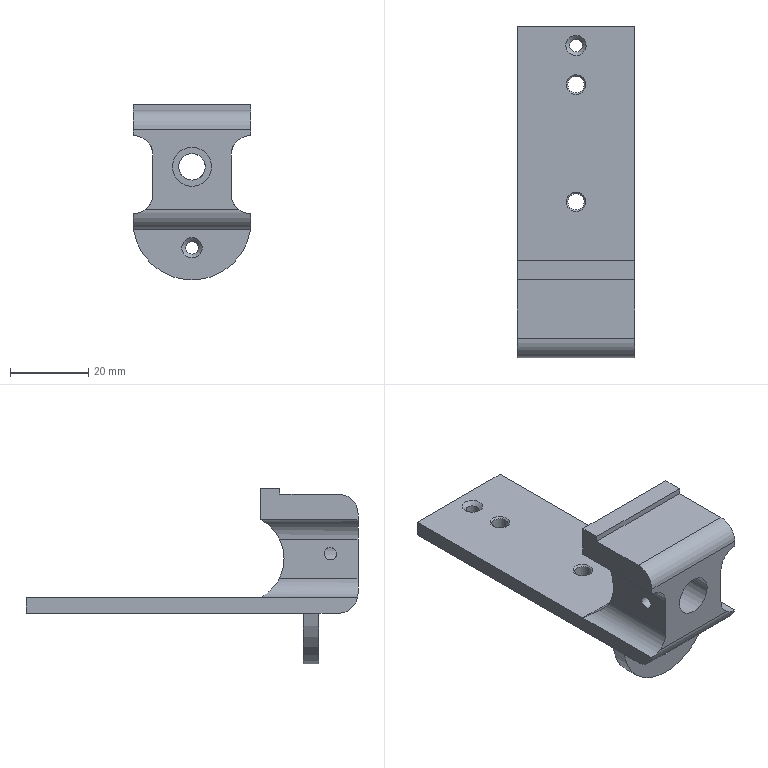Part | NX | features SKETCH 12, EXTRUDE 11, Linear Dimension 2, SIMPLE HOLE 2, SYMBOLIC_THREAD 2, BLEND 1, CHAMFER 1, DATUM_CSYS 1, HOLE PACKAGE 1 | 1 solid | 39 faces | box 30 x 85 x 45 mm | volume 23577 mm3 | plane 18 | cylinder 15 | cone 6 | commonest cylinder face diameters 10 x7 3.2 x3 4.2 x2 6.8 x1 22.545 x1 30.308 x1
STEP:
#1=CARTESIAN_POINT('',(-10.,20.1,-6.25));
#2=VERTEX_POINT('',#1);
#3=CARTESIAN_POINT('',(-10.,20.1,3.75));
#4=VERTEX_POINT('',#3);
#5=CARTESIAN_POINT('',(-10.,30.203,-1.25));
#6=DIRECTION('',(1.,0.,0.));
#7=DIRECTION('',(0.,0.,-1.));
#8=AXIS2_PLACEMENT_3D('',#5,#6,#7);
#9=CIRCLE('',#8,11.273);
#10=EDGE_CURVE('',#2,#4,#9,.F.);
#11=ORIENTED_EDGE('',*,*,#10,.F.);
#12=CARTESIAN_POINT('',(-10.,0.,-6.25));
#13=VERTEX_POINT('',#12);
#14=CARTESIAN_POINT('',(-10.,85.,-6.25));
#15=DIRECTION('',(0.,-1.,0.));
#16=VECTOR('',#15,1000.);
#17=LINE('',#14,#16);
#18=EDGE_CURVE('',#2,#13,#17,.T.);
#19=ORIENTED_EDGE('',*,*,#18,.T.);
#20=CARTESIAN_POINT('',(-10.,0.,3.75));
#21=VERTEX_POINT('',#20);
#22=CARTESIAN_POINT('',(-10.,0.,-6.25));
#23=DIRECTION('',(0.,0.,1.));
#24=VECTOR('',#23,1000.);
#25=LINE('',#22,#24);
#26=EDGE_CURVE('',#13,#21,#25,.T.);
#27=ORIENTED_EDGE('',*,*,#26,.T.);
#28=CARTESIAN_POINT('',(-10.,85.,3.75));
#29=DIRECTION('',(0.,-1.,0.));
#30=VECTOR('',#29,1000.);
#31=LINE('',#28,#30);
#32=EDGE_CURVE('',#4,#21,#31,.T.);
#33=ORIENTED_EDGE('',*,*,#32,.F.);
#34=EDGE_LOOP('',(#11,#19,#27,#33));
#35=FACE_BOUND('',#34,.T.);
#36=CARTESIAN_POINT('',(-10.,5.47,0.));
#37=VERTEX_POINT('',#36);
#38=CARTESIAN_POINT('',(-10.,7.07,0.));
#39=DIRECTION('',(-1.,0.,0.));
#40=DIRECTION('',(0.,-1.,0.));
#41=AXIS2_PLACEMENT_3D('',#38,#39,#40);
#42=CIRCLE('',#41,1.6);
#43=EDGE_CURVE('',#37,#37,#42,.T.);
#44=ORIENTED_EDGE('',*,*,#43,.F.);
#45=EDGE_LOOP('',(#44));
#46=FACE_BOUND('',#45,.T.);
#47=CARTESIAN_POINT('',(-10.,85.,-6.25));
#48=DIRECTION('',(1.,0.,0.));
#49=DIRECTION('',(0.,0.,-1.));
#50=AXIS2_PLACEMENT_3D('',#47,#48,#49);
#51=PLANE('',#50);
#52=ADVANCED_FACE('',(#35,#46),#51,.F.);
#53=CARTESIAN_POINT('',(5.,0.,0.75));
#54=VERTEX_POINT('',#53);
#55=CARTESIAN_POINT('',(0.,0.,0.75));
#56=DIRECTION('',(0.,-1.,0.));
#57=DIRECTION('',(1.,0.,0.));
#58=AXIS2_PLACEMENT_3D('',#55,#56,#57);
#59=CIRCLE('',#58,5.);
#60=EDGE_CURVE('',#54,#54,#59,.T.);
#61=ORIENTED_EDGE('',*,*,#60,.T.);
#62=EDGE_LOOP('',(#61));
#63=FACE_BOUND('',#62,.T.);
#64=CARTESIAN_POINT('',(5.,10.,0.75));
#65=VERTEX_POINT('',#64);
#66=CARTESIAN_POINT('',(0.,10.,0.75));
#67=DIRECTION('',(0.,-1.,0.));
#68=DIRECTION('',(1.,0.,0.));
#69=AXIS2_PLACEMENT_3D('',#66,#67,#68);
#70=CIRCLE('',#69,5.);
#71=EDGE_CURVE('',#65,#65,#70,.T.);
#72=ORIENTED_EDGE('',*,*,#71,.F.);
#73=EDGE_LOOP('',(#72));
#74=FACE_BOUND('',#73,.T.);
#75=CARTESIAN_POINT('',(-4.413,7.07,-1.6));
#76=VERTEX_POINT('',#75);
#77=CARTESIAN_POINT('',(-4.618,8.317,-1.249));
#78=CARTESIAN_POINT('',(-4.311,7.07,-1.776));
#79=CARTESIAN_POINT('',(-4.618,5.821,-1.248));
#80=CARTESIAN_POINT('',(-5.002,5.3,-0.04411));
#81=CARTESIAN_POINT('',(-5.007,5.799,1.248));
#82=CARTESIAN_POINT('',(-4.887,7.069,1.776));
#83=CARTESIAN_POINT('',(-5.007,8.34,1.248));
#84=CARTESIAN_POINT('',(-5.002,8.84,-0.04285));
#85=CARTESIAN_POINT('',(-4.618,8.317,-1.249));
#86=CARTESIAN_POINT('',(-4.311,7.07,-1.776));
#87=CARTESIAN_POINT('',(-4.618,5.821,-1.248));
#88=B_SPLINE_CURVE_WITH_KNOTS('',3,(#77,#78,#79,#80,#81,#82,#83,#84,#85,#86,#87),.UNSPECIFIED.,.T.,.F.,(1,1,1,1,1,1,1,1,1,1,1,1,1,1,1),(-0.003801,-0.002534,-0.001267,0.,0.001267,0.002534,0.003801,0.005068,0.006335,0.007602,0.008869,0.01014,0.0114,0.01267,0.01394),.UNSPECIFIED.);
#89=EDGE_CURVE('',#76,#76,#88,.T.);
#90=ORIENTED_EDGE('',*,*,#89,.T.);
#91=EDGE_LOOP('',(#90));
#92=FACE_BOUND('',#91,.T.);
#93=CARTESIAN_POINT('',(0.,10.,0.75));
#94=DIRECTION('',(0.,-1.,0.));
#95=DIRECTION('',(0.,0.,-1.));
#96=AXIS2_PLACEMENT_3D('',#93,#94,#95);
#97=CYLINDRICAL_SURFACE('',#96,5.);
#98=ADVANCED_FACE('',(#63,#74,#92),#97,.F.);
#99=CARTESIAN_POINT('',(15.,25.,8.75));
#100=VERTEX_POINT('',#99);
#101=CARTESIAN_POINT('',(15.,25.,16.75));
#102=VERTEX_POINT('',#101);
#103=CARTESIAN_POINT('',(15.,25.,-11.25));
#104=DIRECTION('',(0.,0.,1.));
#105=VECTOR('',#104,1000.);
#106=LINE('',#103,#105);
#107=EDGE_CURVE('',#100,#102,#106,.T.);
#108=ORIENTED_EDGE('',*,*,#107,.F.);
#109=CARTESIAN_POINT('',(-15.,25.,8.75));
#110=VERTEX_POINT('',#109);
#111=CARTESIAN_POINT('',(-18.,25.,8.75));
#112=DIRECTION('',(1.,0.,0.));
#113=VECTOR('',#112,1000.);
#114=LINE('',#111,#113);
#115=EDGE_CURVE('',#110,#100,#114,.T.);
#116=ORIENTED_EDGE('',*,*,#115,.F.);
#117=CARTESIAN_POINT('',(-15.,25.,16.75));
#118=VERTEX_POINT('',#117);
#119=CARTESIAN_POINT('',(-15.,25.,16.75));
#120=DIRECTION('',(0.,0.,-1.));
#121=VECTOR('',#120,1000.);
#122=LINE('',#119,#121);
#123=EDGE_CURVE('',#118,#110,#122,.T.);
#124=ORIENTED_EDGE('',*,*,#123,.F.);
#125=CARTESIAN_POINT('',(15.,25.,16.75));
#126=DIRECTION('',(-1.,0.,0.));
#127=VECTOR('',#126,1000.);
#128=LINE('',#125,#127);
#129=EDGE_CURVE('',#102,#118,#128,.T.);
#130=ORIENTED_EDGE('',*,*,#129,.F.);
#131=EDGE_LOOP('',(#108,#116,#124,#130));
#132=FACE_BOUND('',#131,.T.);
#133=CARTESIAN_POINT('',(-18.,25.,-11.25));
#134=DIRECTION('',(0.,1.,0.));
#135=DIRECTION('',(0.,0.,1.));
#136=AXIS2_PLACEMENT_3D('',#133,#134,#135);
#137=PLANE('',#136);
#138=ADVANCED_FACE('',(#132),#137,.T.);
#139=CARTESIAN_POINT('',(10.,20.1,3.75));
#140=VERTEX_POINT('',#139);
#141=CARTESIAN_POINT('',(10.,0.,3.75));
#142=VERTEX_POINT('',#141);
#143=CARTESIAN_POINT('',(10.,85.,3.75));
#144=DIRECTION('',(0.,-1.,0.));
#145=VECTOR('',#144,1000.);
#146=LINE('',#143,#145);
#147=EDGE_CURVE('',#140,#142,#146,.T.);
#148=ORIENTED_EDGE('',*,*,#147,.F.);
#149=CARTESIAN_POINT('',(10.,20.1,3.75));
#150=CARTESIAN_POINT('',(10.,20.45,4.457));
#151=CARTESIAN_POINT('',(10.293,21.285,5.764));
#152=CARTESIAN_POINT('',(11.33,22.76,7.294));
#153=CARTESIAN_POINT('',(12.777,24.25,8.368));
#154=CARTESIAN_POINT('',(14.204,25.,8.75));
#155=CARTESIAN_POINT('',(15.,25.,8.75));
#156=B_SPLINE_CURVE_WITH_KNOTS('',3,(#149,#150,#151,#152,#153,#154,#155),.UNSPECIFIED.,.F.,.F.,(4,1,1,1,4),(0.,0.002329,0.004658,0.006987,0.009316),.UNSPECIFIED.);
#157=EDGE_CURVE('',#140,#100,#156,.T.);
#158=ORIENTED_EDGE('',*,*,#157,.T.);
#159=CARTESIAN_POINT('',(15.,0.,8.75));
#160=VERTEX_POINT('',#159);
#161=CARTESIAN_POINT('',(15.,85.,8.75));
#162=DIRECTION('',(0.,-1.,0.));
#163=VECTOR('',#162,1000.);
#164=LINE('',#161,#163);
#165=EDGE_CURVE('',#100,#160,#164,.T.);
#166=ORIENTED_EDGE('',*,*,#165,.T.);
#167=CARTESIAN_POINT('',(15.,0.,3.75));
#168=DIRECTION('',(0.,1.,0.));
#169=DIRECTION('',(1.,0.,0.));
#170=AXIS2_PLACEMENT_3D('',#167,#168,#169);
#171=CIRCLE('',#170,5.);
#172=EDGE_CURVE('',#142,#160,#171,.T.);
#173=ORIENTED_EDGE('',*,*,#172,.F.);
#174=EDGE_LOOP('',(#148,#158,#166,#173));
#175=FACE_BOUND('',#174,.T.);
#176=CARTESIAN_POINT('',(15.,85.,3.75));
#177=DIRECTION('',(0.,-1.,0.));
#178=DIRECTION('',(0.,0.,-1.));
#179=AXIS2_PLACEMENT_3D('',#176,#177,#178);
#180=CYLINDRICAL_SURFACE('',#179,5.);
#181=ADVANCED_FACE('',(#175),#180,.F.);
#182=CARTESIAN_POINT('',(15.,25.,-11.25));
#183=VERTEX_POINT('',#182);
#184=CARTESIAN_POINT('',(15.,0.101,-11.25));
#185=VERTEX_POINT('',#184);
#186=CARTESIAN_POINT('',(15.,85.,-11.25));
#187=DIRECTION('',(0.,-1.,0.));
#188=VECTOR('',#187,1000.);
#189=LINE('',#186,#188);
#190=EDGE_CURVE('',#183,#185,#189,.T.);
#191=ORIENTED_EDGE('',*,*,#190,.F.);
#192=CARTESIAN_POINT('',(10.,20.1,-6.25));
#193=VERTEX_POINT('',#192);
#194=CARTESIAN_POINT('',(15.,25.,-11.25));
#195=CARTESIAN_POINT('',(14.207,25.,-11.25));
#196=CARTESIAN_POINT('',(12.784,24.255,-10.871));
#197=CARTESIAN_POINT('',(11.33,22.76,-9.795));
#198=CARTESIAN_POINT('',(10.293,21.284,-8.264));
#199=CARTESIAN_POINT('',(10.,20.449,-6.955));
#200=CARTESIAN_POINT('',(10.,20.1,-6.25));
#201=B_SPLINE_CURVE_WITH_KNOTS('',3,(#194,#195,#196,#197,#198,#199,#200),.UNSPECIFIED.,.F.,.F.,(4,1,1,1,4),(0.,0.002339,0.004679,0.007018,0.009357),.UNSPECIFIED.);
#202=EDGE_CURVE('',#183,#193,#201,.T.);
#203=ORIENTED_EDGE('',*,*,#202,.T.);
#204=CARTESIAN_POINT('',(10.,0.,-6.25));
#205=VERTEX_POINT('',#204);
#206=CARTESIAN_POINT('',(10.,85.,-6.25));
#207=DIRECTION('',(0.,-1.,0.));
#208=VECTOR('',#207,1000.);
#209=LINE('',#206,#208);
#210=EDGE_CURVE('',#193,#205,#209,.T.);
#211=ORIENTED_EDGE('',*,*,#210,.T.);
#212=CARTESIAN_POINT('',(12.,0.,-10.25));
#213=VERTEX_POINT('',#212);
#214=CARTESIAN_POINT('',(15.,0.,-6.25));
#215=DIRECTION('',(0.,1.,0.));
#216=DIRECTION('',(1.,0.,0.));
#217=AXIS2_PLACEMENT_3D('',#214,#215,#216);
#218=CIRCLE('',#217,5.);
#219=EDGE_CURVE('',#213,#205,#218,.T.);
#220=ORIENTED_EDGE('',*,*,#219,.F.);
#221=CARTESIAN_POINT('',(12.,0.,-10.25));
#222=CARTESIAN_POINT('',(12.867,0.,-10.9));
#223=CARTESIAN_POINT('',(13.917,0.101,-11.25));
#224=CARTESIAN_POINT('',(15.,0.101,-11.25));
#225=B_SPLINE_CURVE_WITH_KNOTS('',3,(#221,#222,#223,#224),.UNSPECIFIED.,.F.,.F.,(4,4),(0.,0.003202),.UNSPECIFIED.);
#226=EDGE_CURVE('',#213,#185,#225,.T.);
#227=ORIENTED_EDGE('',*,*,#226,.T.);
#228=EDGE_LOOP('',(#191,#203,#211,#220,#227));
#229=FACE_BOUND('',#228,.T.);
#230=CARTESIAN_POINT('',(15.,85.,-6.25));
#231=DIRECTION('',(0.,-1.,0.));
#232=DIRECTION('',(0.,0.,-1.));
#233=AXIS2_PLACEMENT_3D('',#230,#231,#232);
#234=CYLINDRICAL_SURFACE('',#233,5.);
#235=ADVANCED_FACE('',(#229),#234,.F.);
#236=ORIENTED_EDGE('',*,*,#210,.F.);
#237=CARTESIAN_POINT('',(10.,30.203,-1.25));
#238=DIRECTION('',(1.,0.,0.));
#239=DIRECTION('',(0.,0.,-1.));
#240=AXIS2_PLACEMENT_3D('',#237,#238,#239);
#241=CIRCLE('',#240,11.273);
#242=EDGE_CURVE('',#193,#140,#241,.F.);
#243=ORIENTED_EDGE('',*,*,#242,.T.);
#244=ORIENTED_EDGE('',*,*,#147,.T.);
#245=CARTESIAN_POINT('',(10.,0.,-6.25));
#246=DIRECTION('',(0.,0.,1.));
#247=VECTOR('',#246,1000.);
#248=LINE('',#245,#247);
#249=EDGE_CURVE('',#205,#142,#248,.T.);
#250=ORIENTED_EDGE('',*,*,#249,.F.);
#251=EDGE_LOOP('',(#236,#243,#244,#250));
#252=FACE_BOUND('',#251,.T.);
#253=CARTESIAN_POINT('',(10.,85.,-6.25));
#254=DIRECTION('',(1.,0.,0.));
#255=DIRECTION('',(0.,0.,-1.));
#256=AXIS2_PLACEMENT_3D('',#253,#254,#255);
#257=PLANE('',#256);
#258=ADVANCED_FACE('',(#252),#257,.T.);
#259=CARTESIAN_POINT('',(-15.,25.,-11.25));
#260=VERTEX_POINT('',#259);
#261=CARTESIAN_POINT('',(-15.,25.,-11.25));
#262=CARTESIAN_POINT('',(-14.207,25.,-11.25));
#263=CARTESIAN_POINT('',(-12.784,24.255,-10.871));
#264=CARTESIAN_POINT('',(-11.33,22.76,-9.795));
#265=CARTESIAN_POINT('',(-10.293,21.284,-8.264));
#266=CARTESIAN_POINT('',(-10.,20.449,-6.955));
#267=CARTESIAN_POINT('',(-10.,20.1,-6.25));
#268=B_SPLINE_CURVE_WITH_KNOTS('',3,(#261,#262,#263,#264,#265,#266,#267),.UNSPECIFIED.,.F.,.F.,(4,1,1,1,4),(0.,0.002339,0.004679,0.007018,0.009357),.UNSPECIFIED.);
#269=EDGE_CURVE('',#260,#2,#268,.T.);
#270=ORIENTED_EDGE('',*,*,#269,.F.);
#271=CARTESIAN_POINT('',(-15.,0.101,-11.25));
#272=VERTEX_POINT('',#271);
#273=CARTESIAN_POINT('',(-15.,85.,-11.25));
#274=DIRECTION('',(0.,-1.,0.));
#275=VECTOR('',#274,1000.);
#276=LINE('',#273,#275);
#277=EDGE_CURVE('',#260,#272,#276,.T.);
#278=ORIENTED_EDGE('',*,*,#277,.T.);
#279=CARTESIAN_POINT('',(-12.,0.,-10.25));
#280=VERTEX_POINT('',#279);
#281=CARTESIAN_POINT('',(-15.,0.101,-11.25));
#282=CARTESIAN_POINT('',(-13.917,0.101,-11.25));
#283=CARTESIAN_POINT('',(-12.866,0.,-10.9));
#284=CARTESIAN_POINT('',(-12.,0.,-10.25));
#285=B_SPLINE_CURVE_WITH_KNOTS('',3,(#281,#282,#283,#284),.UNSPECIFIED.,.F.,.F.,(4,4),(0.,0.003201),.UNSPECIFIED.);
#286=EDGE_CURVE('',#272,#280,#285,.T.);
#287=ORIENTED_EDGE('',*,*,#286,.T.);
#288=CARTESIAN_POINT('',(-15.,0.,-6.25));
#289=DIRECTION('',(0.,-1.,0.));
#290=DIRECTION('',(1.,0.,0.));
#291=AXIS2_PLACEMENT_3D('',#288,#289,#290);
#292=CIRCLE('',#291,5.);
#293=EDGE_CURVE('',#280,#13,#292,.T.);
#294=ORIENTED_EDGE('',*,*,#293,.T.);
#295=ORIENTED_EDGE('',*,*,#18,.F.);
#296=EDGE_LOOP('',(#270,#278,#287,#294,#295));
#297=FACE_BOUND('',#296,.T.);
#298=CARTESIAN_POINT('',(-15.,85.,-6.25));
#299=DIRECTION('',(0.,-1.,0.));
#300=DIRECTION('',(0.,0.,-1.));
#301=AXIS2_PLACEMENT_3D('',#298,#299,#300);
#302=CYLINDRICAL_SURFACE('',#301,5.);
#303=ADVANCED_FACE('',(#297),#302,.F.);
#304=CARTESIAN_POINT('',(-10.,20.1,3.75));
#305=CARTESIAN_POINT('',(-10.,20.45,4.457));
#306=CARTESIAN_POINT('',(-10.293,21.285,5.764));
#307=CARTESIAN_POINT('',(-11.33,22.76,7.294));
#308=CARTESIAN_POINT('',(-12.777,24.25,8.368));
#309=CARTESIAN_POINT('',(-14.204,25.,8.75));
#310=CARTESIAN_POINT('',(-15.,25.,8.75));
#311=B_SPLINE_CURVE_WITH_KNOTS('',3,(#304,#305,#306,#307,#308,#309,#310),.UNSPECIFIED.,.F.,.F.,(4,1,1,1,4),(0.,0.002329,0.004658,0.006987,0.009316),.UNSPECIFIED.);
#312=EDGE_CURVE('',#4,#110,#311,.T.);
#313=ORIENTED_EDGE('',*,*,#312,.F.);
#314=ORIENTED_EDGE('',*,*,#32,.T.);
#315=CARTESIAN_POINT('',(-15.,0.,8.75));
#316=VERTEX_POINT('',#315);
#317=CARTESIAN_POINT('',(-15.,0.,3.75));
#318=DIRECTION('',(0.,-1.,0.));
#319=DIRECTION('',(1.,0.,0.));
#320=AXIS2_PLACEMENT_3D('',#317,#318,#319);
#321=CIRCLE('',#320,5.);
#322=EDGE_CURVE('',#21,#316,#321,.T.);
#323=ORIENTED_EDGE('',*,*,#322,.T.);
#324=CARTESIAN_POINT('',(-15.,85.,8.75));
#325=DIRECTION('',(0.,-1.,0.));
#326=VECTOR('',#325,1000.);
#327=LINE('',#324,#326);
#328=EDGE_CURVE('',#110,#316,#327,.T.);
#329=ORIENTED_EDGE('',*,*,#328,.F.);
#330=EDGE_LOOP('',(#313,#314,#323,#329));
#331=FACE_BOUND('',#330,.T.);
#332=CARTESIAN_POINT('',(-15.,85.,3.75));
#333=DIRECTION('',(0.,-1.,0.));
#334=DIRECTION('',(0.,0.,-1.));
#335=AXIS2_PLACEMENT_3D('',#332,#333,#334);
#336=CYLINDRICAL_SURFACE('',#335,5.);
#337=ADVANCED_FACE('',(#331),#336,.F.);
#338=CARTESIAN_POINT('',(3.4,10.,0.75));
#339=VERTEX_POINT('',#338);
#340=CARTESIAN_POINT('',(0.,10.,0.75));
#341=DIRECTION('',(0.,-1.,0.));
#342=DIRECTION('',(1.,0.,0.));
#343=AXIS2_PLACEMENT_3D('',#340,#341,#342);
#344=CIRCLE('',#343,3.4);
#345=EDGE_CURVE('',#339,#339,#344,.T.);
#346=ORIENTED_EDGE('',*,*,#345,.T.);
#347=EDGE_LOOP('',(#346));
#348=FACE_BOUND('',#347,.T.);
#349=CARTESIAN_POINT('',(0.,19.018,-2.65));
#350=VERTEX_POINT('',#349);
#351=CARTESIAN_POINT('',(-2.712,18.885,-1.892));
#352=CARTESIAN_POINT('',(0.001244,19.084,-3.028));
#353=CARTESIAN_POINT('',(2.707,18.886,-1.894));
#354=CARTESIAN_POINT('',(3.759,18.994,0.8455));
#355=CARTESIAN_POINT('',(2.652,19.864,3.401));
#356=CARTESIAN_POINT('',(0.008689,20.53,4.524));
#357=CARTESIAN_POINT('',(-2.652,19.865,3.404));
#358=CARTESIAN_POINT('',(-3.758,18.996,0.8528));
#359=CARTESIAN_POINT('',(-2.712,18.885,-1.892));
#360=CARTESIAN_POINT('',(0.001244,19.084,-3.028));
#361=CARTESIAN_POINT('',(2.707,18.886,-1.894));
#362=B_SPLINE_CURVE_WITH_KNOTS('',3,(#351,#352,#353,#354,#355,#356,#357,#358,#359,#360,#361),.UNSPECIFIED.,.T.,.F.,(1,1,1,1,1,1,1,1,1,1,1,1,1,1,1),(-0.00809,-0.005393,-0.002697,0.,0.002697,0.005393,0.00809,0.01079,0.01348,0.01618,0.01888,0.02157,0.02427,0.02697,0.02966),.UNSPECIFIED.);
#363=EDGE_CURVE('',#350,#350,#362,.T.);
#364=ORIENTED_EDGE('',*,*,#363,.F.);
#365=EDGE_LOOP('',(#364));
#366=FACE_BOUND('',#365,.T.);
#367=CARTESIAN_POINT('',(0.,92.5,0.75));
#368=DIRECTION('',(0.,-1.,0.));
#369=DIRECTION('',(0.,0.,-1.));
#370=AXIS2_PLACEMENT_3D('',#367,#368,#369);
#371=CYLINDRICAL_SURFACE('',#370,3.4);
#372=ADVANCED_FACE('',(#348,#366),#371,.F.);
#373=CARTESIAN_POINT('',(15.,14.,-15.25));
#374=VERTEX_POINT('',#373);
#375=CARTESIAN_POINT('',(15.,10.,-15.25));
#376=VERTEX_POINT('',#375);
#377=CARTESIAN_POINT('',(15.,85.,-15.25));
#378=DIRECTION('',(0.,-1.,0.));
#379=VECTOR('',#378,1000.);
#380=LINE('',#377,#379);
#381=EDGE_CURVE('',#374,#376,#380,.T.);
#382=ORIENTED_EDGE('',*,*,#381,.T.);
#383=CARTESIAN_POINT('',(-15.,10.,-15.25));
#384=VERTEX_POINT('',#383);
#385=CARTESIAN_POINT('',(0.,10.,-13.096));
#386=DIRECTION('',(0.,-1.,0.));
#387=DIRECTION('',(0.,0.,-1.));
#388=AXIS2_PLACEMENT_3D('',#385,#386,#387);
#389=CIRCLE('',#388,15.154);
#390=EDGE_CURVE('',#376,#384,#389,.F.);
#391=ORIENTED_EDGE('',*,*,#390,.T.);
#392=CARTESIAN_POINT('',(-15.,14.,-15.25));
#393=VERTEX_POINT('',#392);
#394=CARTESIAN_POINT('',(-15.,85.,-15.25));
#395=DIRECTION('',(0.,-1.,0.));
#396=VECTOR('',#395,1000.);
#397=LINE('',#394,#396);
#398=EDGE_CURVE('',#393,#384,#397,.T.);
#399=ORIENTED_EDGE('',*,*,#398,.F.);
#400=CARTESIAN_POINT('',(0.,14.,-13.096));
#401=DIRECTION('',(0.,1.,0.));
#402=DIRECTION('',(0.,0.,1.));
#403=AXIS2_PLACEMENT_3D('',#400,#401,#402);
#404=CIRCLE('',#403,15.154);
#405=EDGE_CURVE('',#393,#374,#404,.F.);
#406=ORIENTED_EDGE('',*,*,#405,.T.);
#407=EDGE_LOOP('',(#382,#391,#399,#406));
#408=FACE_BOUND('',#407,.T.);
#409=CARTESIAN_POINT('',(0.,85.,-13.096));
#410=DIRECTION('',(0.,-1.,0.));
#411=DIRECTION('',(0.,0.,-1.));
#412=AXIS2_PLACEMENT_3D('',#409,#410,#411);
#413=CYLINDRICAL_SURFACE('',#412,15.154);
#414=ADVANCED_FACE('',(#408),#413,.T.);
#415=ORIENTED_EDGE('',*,*,#60,.F.);
#416=EDGE_LOOP('',(#415));
#417=FACE_BOUND('',#416,.T.);
#418=ORIENTED_EDGE('',*,*,#293,.F.);
#419=CARTESIAN_POINT('',(0.,0.,-10.25));
#420=DIRECTION('',(1.,0.,0.));
#421=VECTOR('',#420,1000.);
#422=LINE('',#419,#421);
#423=EDGE_CURVE('',#280,#213,#422,.T.);
#424=ORIENTED_EDGE('',*,*,#423,.T.);
#425=ORIENTED_EDGE('',*,*,#219,.T.);
#426=ORIENTED_EDGE('',*,*,#249,.T.);
#427=ORIENTED_EDGE('',*,*,#172,.T.);
#428=CARTESIAN_POINT('',(15.,0.,10.25));
#429=VERTEX_POINT('',#428);
#430=CARTESIAN_POINT('',(15.,0.,-15.25));
#431=DIRECTION('',(0.,0.,1.));
#432=VECTOR('',#431,1000.);
#433=LINE('',#430,#432);
#434=EDGE_CURVE('',#160,#429,#433,.T.);
#435=ORIENTED_EDGE('',*,*,#434,.T.);
#436=CARTESIAN_POINT('',(-15.,0.,10.25));
#437=VERTEX_POINT('',#436);
#438=CARTESIAN_POINT('',(0.,0.,10.25));
#439=DIRECTION('',(1.,0.,0.));
#440=VECTOR('',#439,1000.);
#441=LINE('',#438,#440);
#442=EDGE_CURVE('',#429,#437,#441,.F.);
#443=ORIENTED_EDGE('',*,*,#442,.T.);
#444=CARTESIAN_POINT('',(-15.,0.,16.75));
#445=DIRECTION('',(0.,0.,-1.));
#446=VECTOR('',#445,1000.);
#447=LINE('',#444,#446);
#448=EDGE_CURVE('',#437,#316,#447,.T.);
#449=ORIENTED_EDGE('',*,*,#448,.T.);
#450=ORIENTED_EDGE('',*,*,#322,.F.);
#451=ORIENTED_EDGE('',*,*,#26,.F.);
#452=EDGE_LOOP('',(#418,#424,#425,#426,#427,#435,#443,#449,#450,#451));
#453=FACE_BOUND('',#452,.T.);
#454=CARTESIAN_POINT('',(0.,0.,-13.096));
#455=DIRECTION('',(0.,-1.,0.));
#456=DIRECTION('',(0.,0.,-1.));
#457=AXIS2_PLACEMENT_3D('',#454,#455,#456);
#458=PLANE('',#457);
#459=ADVANCED_FACE('',(#417,#453),#458,.T.);
#460=CARTESIAN_POINT('',(-15.,85.,-15.25));
#461=VERTEX_POINT('',#460);
#462=CARTESIAN_POINT('',(15.,85.,-15.25));
#463=VERTEX_POINT('',#462);
#464=CARTESIAN_POINT('',(0.,85.,-15.25));
#465=DIRECTION('',(1.,0.,0.));
#466=VECTOR('',#465,1000.);
#467=LINE('',#464,#466);
#468=EDGE_CURVE('',#461,#463,#467,.T.);
#469=ORIENTED_EDGE('',*,*,#468,.F.);
#470=CARTESIAN_POINT('',(-15.,85.,-11.25));
#471=VERTEX_POINT('',#470);
#472=CARTESIAN_POINT('',(-15.,85.,16.75));
#473=DIRECTION('',(0.,0.,-1.));
#474=VECTOR('',#473,1000.);
#475=LINE('',#472,#474);
#476=EDGE_CURVE('',#471,#461,#475,.T.);
#477=ORIENTED_EDGE('',*,*,#476,.F.);
#478=CARTESIAN_POINT('',(15.,85.,-11.25));
#479=VERTEX_POINT('',#478);
#480=CARTESIAN_POINT('',(0.,85.,-11.25));
#481=DIRECTION('',(-1.,0.,0.));
#482=VECTOR('',#481,1000.);
#483=LINE('',#480,#482);
#484=EDGE_CURVE('',#479,#471,#483,.T.);
#485=ORIENTED_EDGE('',*,*,#484,.F.);
#486=CARTESIAN_POINT('',(15.,85.,-15.25));
#487=DIRECTION('',(0.,0.,1.));
#488=VECTOR('',#487,1000.);
#489=LINE('',#486,#488);
#490=EDGE_CURVE('',#463,#479,#489,.T.);
#491=ORIENTED_EDGE('',*,*,#490,.F.);
#492=EDGE_LOOP('',(#469,#477,#485,#491));
#493=FACE_BOUND('',#492,.T.);
#494=CARTESIAN_POINT('',(0.,85.,-13.096));
#495=DIRECTION('',(0.,-1.,0.));
#496=DIRECTION('',(0.,0.,-1.));
#497=AXIS2_PLACEMENT_3D('',#494,#495,#496);
#498=PLANE('',#497);
#499=ADVANCED_FACE('',(#493),#498,.F.);
#500=CARTESIAN_POINT('',(-15.,5.,-15.25));
#501=VERTEX_POINT('',#500);
#502=CARTESIAN_POINT('',(-15.,85.,-15.25));
#503=DIRECTION('',(0.,-1.,0.));
#504=VECTOR('',#503,1000.);
#505=LINE('',#502,#504);
#506=EDGE_CURVE('',#384,#501,#505,.T.);
#507=ORIENTED_EDGE('',*,*,#506,.T.);
#508=CARTESIAN_POINT('',(-15.,5.,-10.25));
#509=DIRECTION('',(-1.,0.,0.));
#510=DIRECTION('',(0.,0.,1.));
#511=AXIS2_PLACEMENT_3D('',#508,#509,#510);
#512=CIRCLE('',#511,5.);
#513=EDGE_CURVE('',#501,#272,#512,.T.);
#514=ORIENTED_EDGE('',*,*,#513,.T.);
#515=ORIENTED_EDGE('',*,*,#277,.F.);
#516=CARTESIAN_POINT('',(-15.,85.,-11.25));
#517=DIRECTION('',(0.,1.,0.));
#518=VECTOR('',#517,1000.);
#519=LINE('',#516,#518);
#520=EDGE_CURVE('',#260,#471,#519,.T.);
#521=ORIENTED_EDGE('',*,*,#520,.T.);
#522=ORIENTED_EDGE('',*,*,#476,.T.);
#523=CARTESIAN_POINT('',(-15.,85.,-15.25));
#524=DIRECTION('',(0.,-1.,0.));
#525=VECTOR('',#524,1000.);
#526=LINE('',#523,#525);
#527=EDGE_CURVE('',#461,#393,#526,.T.);
#528=ORIENTED_EDGE('',*,*,#527,.T.);
#529=ORIENTED_EDGE('',*,*,#398,.T.);
#530=EDGE_LOOP('',(#507,#514,#515,#521,#522,#528,#529));
#531=FACE_BOUND('',#530,.T.);
#532=CARTESIAN_POINT('',(-15.,85.,16.75));
#533=DIRECTION('',(-1.,0.,0.));
#534=DIRECTION('',(0.,0.,1.));
#535=AXIS2_PLACEMENT_3D('',#532,#533,#534);
#536=PLANE('',#535);
#537=ADVANCED_FACE('',(#531),#536,.T.);
#538=CARTESIAN_POINT('',(15.,20.,15.25));
#539=VERTEX_POINT('',#538);
#540=CARTESIAN_POINT('',(15.,5.,15.25));
#541=VERTEX_POINT('',#540);
#542=CARTESIAN_POINT('',(15.,20.,15.25));
#543=DIRECTION('',(0.,-1.,0.));
#544=VECTOR('',#543,1000.);
#545=LINE('',#542,#544);
#546=EDGE_CURVE('',#539,#541,#545,.T.);
#547=ORIENTED_EDGE('',*,*,#546,.T.);
#548=CARTESIAN_POINT('',(15.,5.,10.25));
#549=DIRECTION('',(1.,0.,0.));
#550=DIRECTION('',(0.,0.,-1.));
#551=AXIS2_PLACEMENT_3D('',#548,#549,#550);
#552=CIRCLE('',#551,5.);
#553=EDGE_CURVE('',#541,#429,#552,.T.);
#554=ORIENTED_EDGE('',*,*,#553,.T.);
#555=ORIENTED_EDGE('',*,*,#434,.F.);
#556=ORIENTED_EDGE('',*,*,#165,.F.);
#557=ORIENTED_EDGE('',*,*,#107,.T.);
#558=CARTESIAN_POINT('',(15.,20.,16.75));
#559=VERTEX_POINT('',#558);
#560=CARTESIAN_POINT('',(15.,85.,16.75));
#561=DIRECTION('',(0.,-1.,0.));
#562=VECTOR('',#561,1000.);
#563=LINE('',#560,#562);
#564=EDGE_CURVE('',#102,#559,#563,.T.);
#565=ORIENTED_EDGE('',*,*,#564,.T.);
#566=CARTESIAN_POINT('',(15.,20.,16.75));
#567=DIRECTION('',(0.,0.,-1.));
#568=VECTOR('',#567,1000.);
#569=LINE('',#566,#568);
#570=EDGE_CURVE('',#559,#539,#569,.T.);
#571=ORIENTED_EDGE('',*,*,#570,.T.);
#572=EDGE_LOOP('',(#547,#554,#555,#556,#557,#565,#571));
#573=FACE_BOUND('',#572,.T.);
#574=CARTESIAN_POINT('',(15.,85.,-15.25));
#575=DIRECTION('',(1.,0.,0.));
#576=DIRECTION('',(0.,0.,-1.));
#577=AXIS2_PLACEMENT_3D('',#574,#575,#576);
#578=PLANE('',#577);
#579=ADVANCED_FACE('',(#573),#578,.T.);
#580=ORIENTED_EDGE('',*,*,#190,.T.);
#581=CARTESIAN_POINT('',(15.,5.,-15.25));
#582=VERTEX_POINT('',#581);
#583=CARTESIAN_POINT('',(15.,5.,-10.25));
#584=DIRECTION('',(1.,0.,0.));
#585=DIRECTION('',(0.,0.,-1.));
#586=AXIS2_PLACEMENT_3D('',#583,#584,#585);
#587=CIRCLE('',#586,5.);
#588=EDGE_CURVE('',#185,#582,#587,.T.);
#589=ORIENTED_EDGE('',*,*,#588,.T.);
#590=CARTESIAN_POINT('',(15.,-14.,-15.25));
#591=DIRECTION('',(0.,1.,0.));
#592=VECTOR('',#591,1000.);
#593=LINE('',#590,#592);
#594=EDGE_CURVE('',#582,#376,#593,.T.);
#595=ORIENTED_EDGE('',*,*,#594,.T.);
#596=ORIENTED_EDGE('',*,*,#381,.F.);
#597=CARTESIAN_POINT('',(15.,85.,-15.25));
#598=DIRECTION('',(0.,-1.,0.));
#599=VECTOR('',#598,1000.);
#600=LINE('',#597,#599);
#601=EDGE_CURVE('',#463,#374,#600,.T.);
#602=ORIENTED_EDGE('',*,*,#601,.F.);
#603=ORIENTED_EDGE('',*,*,#490,.T.);
#604=CARTESIAN_POINT('',(15.,96.5,-11.25));
#605=DIRECTION('',(0.,-1.,0.));
#606=VECTOR('',#605,1000.);
#607=LINE('',#604,#606);
#608=EDGE_CURVE('',#479,#183,#607,.T.);
#609=ORIENTED_EDGE('',*,*,#608,.T.);
#610=EDGE_LOOP('',(#580,#589,#595,#596,#602,#603,#609));
#611=FACE_BOUND('',#610,.T.);
#612=CARTESIAN_POINT('',(15.,85.,-15.25));
#613=DIRECTION('',(1.,0.,0.));
#614=DIRECTION('',(0.,0.,-1.));
#615=AXIS2_PLACEMENT_3D('',#612,#613,#614);
#616=PLANE('',#615);
#617=ADVANCED_FACE('',(#611),#616,.T.);
#618=ORIENTED_EDGE('',*,*,#448,.F.);
#619=CARTESIAN_POINT('',(-15.,5.,15.25));
#620=VERTEX_POINT('',#619);
#621=CARTESIAN_POINT('',(-15.,5.,10.25));
#622=DIRECTION('',(-1.,0.,0.));
#623=DIRECTION('',(0.,0.,1.));
#624=AXIS2_PLACEMENT_3D('',#621,#622,#623);
#625=CIRCLE('',#624,5.);
#626=EDGE_CURVE('',#437,#620,#625,.T.);
#627=ORIENTED_EDGE('',*,*,#626,.T.);
#628=CARTESIAN_POINT('',(-15.,20.,15.25));
#629=VERTEX_POINT('',#628);
#630=CARTESIAN_POINT('',(-15.,85.,15.25));
#631=DIRECTION('',(0.,1.,0.));
#632=VECTOR('',#631,1000.);
#633=LINE('',#630,#632);
#634=EDGE_CURVE('',#620,#629,#633,.T.);
#635=ORIENTED_EDGE('',*,*,#634,.T.);
#636=CARTESIAN_POINT('',(-15.,20.,16.75));
#637=VERTEX_POINT('',#636);
#638=CARTESIAN_POINT('',(-15.,20.,16.75));
#639=DIRECTION('',(0.,0.,1.));
#640=VECTOR('',#639,1000.);
#641=LINE('',#638,#640);
#642=EDGE_CURVE('',#629,#637,#641,.T.);
#643=ORIENTED_EDGE('',*,*,#642,.T.);
#644=CARTESIAN_POINT('',(-15.,85.,16.75));
#645=DIRECTION('',(0.,-1.,0.));
#646=VECTOR('',#645,1000.);
#647=LINE('',#644,#646);
#648=EDGE_CURVE('',#118,#637,#647,.T.);
#649=ORIENTED_EDGE('',*,*,#648,.F.);
#650=ORIENTED_EDGE('',*,*,#123,.T.);
#651=ORIENTED_EDGE('',*,*,#328,.T.);
#652=EDGE_LOOP('',(#618,#627,#635,#643,#649,#650,#651));
#653=FACE_BOUND('',#652,.T.);
#654=CARTESIAN_POINT('',(-15.,85.,16.75));
#655=DIRECTION('',(-1.,0.,0.));
#656=DIRECTION('',(0.,0.,1.));
#657=AXIS2_PLACEMENT_3D('',#654,#655,#656);
#658=PLANE('',#657);
#659=ADVANCED_FACE('',(#653),#658,.T.);
#660=ORIENTED_EDGE('',*,*,#564,.F.);
#661=ORIENTED_EDGE('',*,*,#129,.T.);
#662=ORIENTED_EDGE('',*,*,#648,.T.);
#663=CARTESIAN_POINT('',(-18.,20.,16.75));
#664=DIRECTION('',(1.,0.,0.));
#665=VECTOR('',#664,1000.);
#666=LINE('',#663,#665);
#667=EDGE_CURVE('',#637,#559,#666,.T.);
#668=ORIENTED_EDGE('',*,*,#667,.T.);
#669=EDGE_LOOP('',(#660,#661,#662,#668));
#670=FACE_BOUND('',#669,.T.);
#671=CARTESIAN_POINT('',(15.,85.,16.75));
#672=DIRECTION('',(0.,0.,1.));
#673=DIRECTION('',(1.,0.,0.));
#674=AXIS2_PLACEMENT_3D('',#671,#672,#673);
#675=PLANE('',#674);
#676=ADVANCED_FACE('',(#670),#675,.T.);
#677=CARTESIAN_POINT('',(-18.,20.,15.25));
#678=DIRECTION('',(1.,0.,0.));
#679=VECTOR('',#678,1000.);
#680=LINE('',#677,#679);
#681=EDGE_CURVE('',#629,#539,#680,.T.);
#682=ORIENTED_EDGE('',*,*,#681,.T.);
#683=ORIENTED_EDGE('',*,*,#570,.F.);
#684=ORIENTED_EDGE('',*,*,#667,.F.);
#685=ORIENTED_EDGE('',*,*,#642,.F.);
#686=EDGE_LOOP('',(#682,#683,#684,#685));
#687=FACE_BOUND('',#686,.T.);
#688=CARTESIAN_POINT('',(-18.,20.,16.75));
#689=DIRECTION('',(0.,-1.,0.));
#690=DIRECTION('',(0.,0.,-1.));
#691=AXIS2_PLACEMENT_3D('',#688,#689,#690);
#692=PLANE('',#691);
#693=ADVANCED_FACE('',(#687),#692,.T.);
#694=ORIENTED_EDGE('',*,*,#634,.F.);
#695=CARTESIAN_POINT('',(-18.,5.,15.25));
#696=DIRECTION('',(1.,0.,0.));
#697=VECTOR('',#696,1000.);
#698=LINE('',#695,#697);
#699=EDGE_CURVE('',#620,#541,#698,.T.);
#700=ORIENTED_EDGE('',*,*,#699,.T.);
#701=ORIENTED_EDGE('',*,*,#546,.F.);
#702=ORIENTED_EDGE('',*,*,#681,.F.);
#703=EDGE_LOOP('',(#694,#700,#701,#702));
#704=FACE_BOUND('',#703,.T.);
#705=CARTESIAN_POINT('',(-18.,20.,15.25));
#706=DIRECTION('',(0.,0.,1.));
#707=DIRECTION('',(0.,-1.,0.));
#708=AXIS2_PLACEMENT_3D('',#705,#706,#707);
#709=PLANE('',#708);
#710=ADVANCED_FACE('',(#704),#709,.T.);
#711=CARTESIAN_POINT('',(0.,67.5,-11.25));
#712=VERTEX_POINT('',#711);
#713=CARTESIAN_POINT('',(0.,70.,-11.25));
#714=DIRECTION('',(0.,0.,1.));
#715=DIRECTION('',(0.,-1.,0.));
#716=AXIS2_PLACEMENT_3D('',#713,#714,#715);
#717=CIRCLE('',#716,2.5);
#718=EDGE_CURVE('',#712,#712,#717,.F.);
#719=ORIENTED_EDGE('',*,*,#718,.T.);
#720=EDGE_LOOP('',(#719));
#721=FACE_BOUND('',#720,.T.);
#722=CARTESIAN_POINT('',(0.,37.5,-11.25));
#723=VERTEX_POINT('',#722);
#724=CARTESIAN_POINT('',(0.,40.,-11.25));
#725=DIRECTION('',(0.,0.,1.));
#726=DIRECTION('',(0.,-1.,0.));
#727=AXIS2_PLACEMENT_3D('',#724,#725,#726);
#728=CIRCLE('',#727,2.5);
#729=EDGE_CURVE('',#723,#723,#728,.F.);
#730=ORIENTED_EDGE('',*,*,#729,.T.);
#731=EDGE_LOOP('',(#730));
#732=FACE_BOUND('',#731,.T.);
#733=CARTESIAN_POINT('',(0.,77.4,-11.25));
#734=VERTEX_POINT('',#733);
#735=CARTESIAN_POINT('',(0.,80.,-11.25));
#736=DIRECTION('',(0.,0.,1.));
#737=DIRECTION('',(0.,-1.,0.));
#738=AXIS2_PLACEMENT_3D('',#735,#736,#737);
#739=CIRCLE('',#738,2.6);
#740=EDGE_CURVE('',#734,#734,#739,.F.);
#741=ORIENTED_EDGE('',*,*,#740,.T.);
#742=EDGE_LOOP('',(#741));
#743=FACE_BOUND('',#742,.T.);
#744=CARTESIAN_POINT('',(-18.,25.,-11.25));
#745=DIRECTION('',(1.,0.,0.));
#746=VECTOR('',#745,1000.);
#747=LINE('',#744,#746);
#748=EDGE_CURVE('',#260,#183,#747,.T.);
#749=ORIENTED_EDGE('',*,*,#748,.T.);
#750=ORIENTED_EDGE('',*,*,#608,.F.);
#751=ORIENTED_EDGE('',*,*,#484,.T.);
#752=ORIENTED_EDGE('',*,*,#520,.F.);
#753=EDGE_LOOP('',(#749,#750,#751,#752));
#754=FACE_BOUND('',#753,.T.);
#755=CARTESIAN_POINT('',(-18.,96.5,-11.25));
#756=DIRECTION('',(0.,0.,1.));
#757=DIRECTION('',(0.,-1.,0.));
#758=AXIS2_PLACEMENT_3D('',#755,#756,#757);
#759=PLANE('',#758);
#760=ADVANCED_FACE('',(#721,#732,#743,#754),#759,.T.);
#761=CARTESIAN_POINT('',(-2.5,70.,-15.25));
#762=VERTEX_POINT('',#761);
#763=CARTESIAN_POINT('',(0.,70.,-15.25));
#764=DIRECTION('',(0.,0.,-1.));
#765=DIRECTION('',(-1.,0.,0.));
#766=AXIS2_PLACEMENT_3D('',#763,#764,#765);
#767=CIRCLE('',#766,2.5);
#768=EDGE_CURVE('',#762,#762,#767,.F.);
#769=ORIENTED_EDGE('',*,*,#768,.T.);
#770=EDGE_LOOP('',(#769));
#771=FACE_BOUND('',#770,.T.);
#772=CARTESIAN_POINT('',(-2.5,40.,-15.25));
#773=VERTEX_POINT('',#772);
#774=CARTESIAN_POINT('',(0.,40.,-15.25));
#775=DIRECTION('',(0.,0.,-1.));
#776=DIRECTION('',(-1.,0.,0.));
#777=AXIS2_PLACEMENT_3D('',#774,#775,#776);
#778=CIRCLE('',#777,2.5);
#779=EDGE_CURVE('',#773,#773,#778,.F.);
#780=ORIENTED_EDGE('',*,*,#779,.T.);
#781=EDGE_LOOP('',(#780));
#782=FACE_BOUND('',#781,.T.);
#783=CARTESIAN_POINT('',(-1.6,80.,-15.25));
#784=VERTEX_POINT('',#783);
#785=CARTESIAN_POINT('',(0.,80.,-15.25));
#786=DIRECTION('',(0.,0.,-1.));
#787=DIRECTION('',(-1.,0.,0.));
#788=AXIS2_PLACEMENT_3D('',#785,#786,#787);
#789=CIRCLE('',#788,1.6);
#790=EDGE_CURVE('',#784,#784,#789,.T.);
#791=ORIENTED_EDGE('',*,*,#790,.F.);
#792=EDGE_LOOP('',(#791));
#793=FACE_BOUND('',#792,.T.);
#794=ORIENTED_EDGE('',*,*,#468,.T.);
#795=ORIENTED_EDGE('',*,*,#601,.T.);
#796=CARTESIAN_POINT('',(-18.,14.,-15.25));
#797=DIRECTION('',(1.,0.,0.));
#798=VECTOR('',#797,1000.);
#799=LINE('',#796,#798);
#800=EDGE_CURVE('',#393,#374,#799,.T.);
#801=ORIENTED_EDGE('',*,*,#800,.F.);
#802=ORIENTED_EDGE('',*,*,#527,.F.);
#803=EDGE_LOOP('',(#794,#795,#801,#802));
#804=FACE_BOUND('',#803,.T.);
#805=CARTESIAN_POINT('',(-18.,14.,-15.25));
#806=DIRECTION('',(0.,0.,-1.));
#807=DIRECTION('',(-1.,0.,0.));
#808=AXIS2_PLACEMENT_3D('',#805,#806,#807);
#809=PLANE('',#808);
#810=ADVANCED_FACE('',(#771,#782,#793,#804),#809,.T.);
#811=CARTESIAN_POINT('',(0.,14.,-18.4));
#812=VERTEX_POINT('',#811);
#813=CARTESIAN_POINT('',(0.,14.,-20.));
#814=DIRECTION('',(0.,1.,0.));
#815=DIRECTION('',(0.,0.,1.));
#816=AXIS2_PLACEMENT_3D('',#813,#814,#815);
#817=CIRCLE('',#816,1.6);
#818=EDGE_CURVE('',#812,#812,#817,.T.);
#819=ORIENTED_EDGE('',*,*,#818,.F.);
#820=EDGE_LOOP('',(#819));
#821=FACE_BOUND('',#820,.T.);
#822=ORIENTED_EDGE('',*,*,#800,.T.);
#823=ORIENTED_EDGE('',*,*,#405,.F.);
#824=EDGE_LOOP('',(#822,#823));
#825=FACE_BOUND('',#824,.T.);
#826=CARTESIAN_POINT('',(-18.,14.,-38.75));
#827=DIRECTION('',(0.,1.,0.));
#828=DIRECTION('',(0.,0.,1.));
#829=AXIS2_PLACEMENT_3D('',#826,#827,#828);
#830=PLANE('',#829);
#831=ADVANCED_FACE('',(#821,#825),#830,.T.);
#832=ORIENTED_EDGE('',*,*,#594,.F.);
#833=CARTESIAN_POINT('',(-18.,5.,-15.25));
#834=DIRECTION('',(1.,0.,0.));
#835=VECTOR('',#834,1000.);
#836=LINE('',#833,#835);
#837=EDGE_CURVE('',#582,#501,#836,.F.);
#838=ORIENTED_EDGE('',*,*,#837,.T.);
#839=ORIENTED_EDGE('',*,*,#506,.F.);
#840=CARTESIAN_POINT('',(-18.,10.,-15.25));
#841=DIRECTION('',(1.,0.,0.));
#842=VECTOR('',#841,1000.);
#843=LINE('',#840,#842);
#844=EDGE_CURVE('',#384,#376,#843,.T.);
#845=ORIENTED_EDGE('',*,*,#844,.T.);
#846=EDGE_LOOP('',(#832,#838,#839,#845));
#847=FACE_BOUND('',#846,.T.);
#848=CARTESIAN_POINT('',(-18.,-14.,-15.25));
#849=DIRECTION('',(0.,0.,-1.));
#850=DIRECTION('',(-1.,0.,0.));
#851=AXIS2_PLACEMENT_3D('',#848,#849,#850);
#852=PLANE('',#851);
#853=ADVANCED_FACE('',(#847),#852,.T.);
#854=CARTESIAN_POINT('',(0.,10.,-22.6));
#855=VERTEX_POINT('',#854);
#856=CARTESIAN_POINT('',(0.,10.,-20.));
#857=DIRECTION('',(0.,-1.,0.));
#858=DIRECTION('',(0.,0.,-1.));
#859=AXIS2_PLACEMENT_3D('',#856,#857,#858);
#860=CIRCLE('',#859,2.6);
#861=EDGE_CURVE('',#855,#855,#860,.F.);
#862=ORIENTED_EDGE('',*,*,#861,.T.);
#863=EDGE_LOOP('',(#862));
#864=FACE_BOUND('',#863,.T.);
#865=ORIENTED_EDGE('',*,*,#844,.F.);
#866=ORIENTED_EDGE('',*,*,#390,.F.);
#867=EDGE_LOOP('',(#865,#866));
#868=FACE_BOUND('',#867,.T.);
#869=CARTESIAN_POINT('',(-18.,10.,-15.25));
#870=DIRECTION('',(0.,-1.,0.));
#871=DIRECTION('',(0.,0.,-1.));
#872=AXIS2_PLACEMENT_3D('',#869,#870,#871);
#873=PLANE('',#872);
#874=ADVANCED_FACE('',(#864,#868),#873,.T.);
#875=ORIENTED_EDGE('',*,*,#513,.F.);
#876=ORIENTED_EDGE('',*,*,#837,.F.);
#877=ORIENTED_EDGE('',*,*,#588,.F.);
#878=ORIENTED_EDGE('',*,*,#226,.F.);
#879=ORIENTED_EDGE('',*,*,#423,.F.);
#880=ORIENTED_EDGE('',*,*,#286,.F.);
#881=EDGE_LOOP('',(#875,#876,#877,#878,#879,#880));
#882=FACE_BOUND('',#881,.T.);
#883=CARTESIAN_POINT('',(0.,5.,-10.25));
#884=DIRECTION('',(1.,0.,0.));
#885=DIRECTION('',(0.,0.,-1.));
#886=AXIS2_PLACEMENT_3D('',#883,#884,#885);
#887=CYLINDRICAL_SURFACE('',#886,5.);
#888=ADVANCED_FACE('',(#882),#887,.T.);
#889=ORIENTED_EDGE('',*,*,#626,.F.);
#890=ORIENTED_EDGE('',*,*,#442,.F.);
#891=ORIENTED_EDGE('',*,*,#553,.F.);
#892=ORIENTED_EDGE('',*,*,#699,.F.);
#893=EDGE_LOOP('',(#889,#890,#891,#892));
#894=FACE_BOUND('',#893,.T.);
#895=CARTESIAN_POINT('',(-18.,5.,10.25));
#896=DIRECTION('',(1.,0.,0.));
#897=DIRECTION('',(0.,0.,-1.));
#898=AXIS2_PLACEMENT_3D('',#895,#896,#897);
#899=CYLINDRICAL_SURFACE('',#898,5.);
#900=ADVANCED_FACE('',(#894),#899,.T.);
#901=ORIENTED_EDGE('',*,*,#345,.F.);
#902=EDGE_LOOP('',(#901));
#903=FACE_BOUND('',#902,.T.);
#904=ORIENTED_EDGE('',*,*,#71,.T.);
#905=EDGE_LOOP('',(#904));
#906=FACE_BOUND('',#905,.T.);
#907=CARTESIAN_POINT('',(0.,10.,0.));
#908=DIRECTION('',(0.,-1.,0.));
#909=DIRECTION('',(0.,0.,-1.));
#910=AXIS2_PLACEMENT_3D('',#907,#908,#909);
#911=PLANE('',#910);
#912=ADVANCED_FACE('',(#903,#906),#911,.T.);
#913=CARTESIAN_POINT('',(1.6,80.,-12.25));
#914=VERTEX_POINT('',#913);
#915=CARTESIAN_POINT('',(0.,80.,-12.25));
#916=DIRECTION('',(0.,0.,1.));
#917=DIRECTION('',(1.,0.,0.));
#918=AXIS2_PLACEMENT_3D('',#915,#916,#917);
#919=CIRCLE('',#918,1.6);
#920=EDGE_CURVE('',#914,#914,#919,.T.);
#921=ORIENTED_EDGE('',*,*,#920,.T.);
#922=EDGE_LOOP('',(#921));
#923=FACE_BOUND('',#922,.T.);
#924=ORIENTED_EDGE('',*,*,#790,.T.);
#925=EDGE_LOOP('',(#924));
#926=FACE_BOUND('',#925,.T.);
#927=CARTESIAN_POINT('',(0.,80.,-21.25));
#928=DIRECTION('',(0.,0.,1.));
#929=DIRECTION('',(1.,0.,0.));
#930=AXIS2_PLACEMENT_3D('',#927,#928,#929);
#931=CYLINDRICAL_SURFACE('',#930,1.6);
#932=ADVANCED_FACE('',(#923,#926),#931,.F.);
#933=CARTESIAN_POINT('',(0.,11.,-21.6));
#934=VERTEX_POINT('',#933);
#935=CARTESIAN_POINT('',(0.,11.,-20.));
#936=DIRECTION('',(0.,-1.,0.));
#937=DIRECTION('',(0.,0.,-1.));
#938=AXIS2_PLACEMENT_3D('',#935,#936,#937);
#939=CIRCLE('',#938,1.6);
#940=EDGE_CURVE('',#934,#934,#939,.T.);
#941=ORIENTED_EDGE('',*,*,#940,.T.);
#942=EDGE_LOOP('',(#941));
#943=FACE_BOUND('',#942,.T.);
#944=ORIENTED_EDGE('',*,*,#818,.T.);
#945=EDGE_LOOP('',(#944));
#946=FACE_BOUND('',#945,.T.);
#947=CARTESIAN_POINT('',(0.,20.,-20.));
#948=DIRECTION('',(0.,-1.,0.));
#949=DIRECTION('',(0.,0.,-1.));
#950=AXIS2_PLACEMENT_3D('',#947,#948,#949);
#951=CYLINDRICAL_SURFACE('',#950,1.6);
#952=ADVANCED_FACE('',(#943,#946),#951,.F.);
#953=ORIENTED_EDGE('',*,*,#861,.F.);
#954=EDGE_LOOP('',(#953));
#955=FACE_BOUND('',#954,.T.);
#956=ORIENTED_EDGE('',*,*,#940,.F.);
#957=EDGE_LOOP('',(#956));
#958=FACE_BOUND('',#957,.T.);
#959=CARTESIAN_POINT('',(0.,11.,-20.));
#960=DIRECTION('',(0.,-1.,0.));
#961=DIRECTION('',(0.,0.,-1.));
#962=AXIS2_PLACEMENT_3D('',#959,#960,#961);
#963=CONICAL_SURFACE('',#962,1.6,0.7854);
#964=ADVANCED_FACE('',(#955,#958),#963,.F.);
#965=ORIENTED_EDGE('',*,*,#740,.F.);
#966=EDGE_LOOP('',(#965));
#967=FACE_BOUND('',#966,.T.);
#968=ORIENTED_EDGE('',*,*,#920,.F.);
#969=EDGE_LOOP('',(#968));
#970=FACE_BOUND('',#969,.T.);
#971=CARTESIAN_POINT('',(0.,80.,-12.25));
#972=DIRECTION('',(0.,0.,1.));
#973=DIRECTION('',(1.,0.,0.));
#974=AXIS2_PLACEMENT_3D('',#971,#972,#973);
#975=CONICAL_SURFACE('',#974,1.6,0.7854);
#976=ADVANCED_FACE('',(#967,#970),#975,.F.);
#977=CARTESIAN_POINT('',(-2.1,40.,-14.85));
#978=VERTEX_POINT('',#977);
#979=CARTESIAN_POINT('',(0.,40.,-14.85));
#980=DIRECTION('',(0.,0.,-1.));
#981=DIRECTION('',(-1.,0.,0.));
#982=AXIS2_PLACEMENT_3D('',#979,#980,#981);
#983=CIRCLE('',#982,2.1);
#984=EDGE_CURVE('',#978,#978,#983,.T.);
#985=ORIENTED_EDGE('',*,*,#984,.T.);
#986=EDGE_LOOP('',(#985));
#987=FACE_BOUND('',#986,.T.);
#988=CARTESIAN_POINT('',(2.1,40.,-11.65));
#989=VERTEX_POINT('',#988);
#990=CARTESIAN_POINT('',(0.,40.,-11.65));
#991=DIRECTION('',(0.,0.,1.));
#992=DIRECTION('',(1.,0.,0.));
#993=AXIS2_PLACEMENT_3D('',#990,#991,#992);
#994=CIRCLE('',#993,2.1);
#995=EDGE_CURVE('',#989,#989,#994,.T.);
#996=ORIENTED_EDGE('',*,*,#995,.T.);
#997=EDGE_LOOP('',(#996));
#998=FACE_BOUND('',#997,.T.);
#999=CARTESIAN_POINT('',(0.,40.,-11.25));
#1000=DIRECTION('',(0.,0.,-1.));
#1001=DIRECTION('',(0.,1.,0.));
#1002=AXIS2_PLACEMENT_3D('',#999,#1000,#1001);
#1003=CYLINDRICAL_SURFACE('',#1002,2.1);
#1004=ADVANCED_FACE('',(#987,#998),#1003,.F.);
#1005=ORIENTED_EDGE('',*,*,#995,.F.);
#1006=EDGE_LOOP('',(#1005));
#1007=FACE_BOUND('',#1006,.T.);
#1008=ORIENTED_EDGE('',*,*,#729,.F.);
#1009=EDGE_LOOP('',(#1008));
#1010=FACE_BOUND('',#1009,.T.);
#1011=CARTESIAN_POINT('',(0.,40.,-11.25));
#1012=DIRECTION('',(0.,0.,1.));
#1013=DIRECTION('',(1.,0.,0.));
#1014=AXIS2_PLACEMENT_3D('',#1011,#1012,#1013);
#1015=CONICAL_SURFACE('',#1014,2.5,0.7854);
#1016=ADVANCED_FACE('',(#1007,#1010),#1015,.F.);
#1017=ORIENTED_EDGE('',*,*,#779,.F.);
#1018=EDGE_LOOP('',(#1017));
#1019=FACE_BOUND('',#1018,.T.);
#1020=ORIENTED_EDGE('',*,*,#984,.F.);
#1021=EDGE_LOOP('',(#1020));
#1022=FACE_BOUND('',#1021,.T.);
#1023=CARTESIAN_POINT('',(0.,40.,-14.85));
#1024=DIRECTION('',(0.,0.,-1.));
#1025=DIRECTION('',(-1.,0.,0.));
#1026=AXIS2_PLACEMENT_3D('',#1023,#1024,#1025);
#1027=CONICAL_SURFACE('',#1026,2.1,0.7854);
#1028=ADVANCED_FACE('',(#1019,#1022),#1027,.F.);
#1029=CARTESIAN_POINT('',(-2.1,70.,-14.85));
#1030=VERTEX_POINT('',#1029);
#1031=CARTESIAN_POINT('',(0.,70.,-14.85));
#1032=DIRECTION('',(0.,0.,-1.));
#1033=DIRECTION('',(-1.,0.,0.));
#1034=AXIS2_PLACEMENT_3D('',#1031,#1032,#1033);
#1035=CIRCLE('',#1034,2.1);
#1036=EDGE_CURVE('',#1030,#1030,#1035,.T.);
#1037=ORIENTED_EDGE('',*,*,#1036,.T.);
#1038=EDGE_LOOP('',(#1037));
#1039=FACE_BOUND('',#1038,.T.);
#1040=CARTESIAN_POINT('',(2.1,70.,-11.65));
#1041=VERTEX_POINT('',#1040);
#1042=CARTESIAN_POINT('',(0.,70.,-11.65));
#1043=DIRECTION('',(0.,0.,1.));
#1044=DIRECTION('',(1.,0.,0.));
#1045=AXIS2_PLACEMENT_3D('',#1042,#1043,#1044);
#1046=CIRCLE('',#1045,2.1);
#1047=EDGE_CURVE('',#1041,#1041,#1046,.T.);
#1048=ORIENTED_EDGE('',*,*,#1047,.T.);
#1049=EDGE_LOOP('',(#1048));
#1050=FACE_BOUND('',#1049,.T.);
#1051=CARTESIAN_POINT('',(0.,70.,-11.25));
#1052=DIRECTION('',(0.,0.,-1.));
#1053=DIRECTION('',(0.,1.,0.));
#1054=AXIS2_PLACEMENT_3D('',#1051,#1052,#1053);
#1055=CYLINDRICAL_SURFACE('',#1054,2.1);
#1056=ADVANCED_FACE('',(#1039,#1050),#1055,.F.);
#1057=ORIENTED_EDGE('',*,*,#1047,.F.);
#1058=EDGE_LOOP('',(#1057));
#1059=FACE_BOUND('',#1058,.T.);
#1060=ORIENTED_EDGE('',*,*,#718,.F.);
#1061=EDGE_LOOP('',(#1060));
#1062=FACE_BOUND('',#1061,.T.);
#1063=CARTESIAN_POINT('',(0.,70.,-11.25));
#1064=DIRECTION('',(0.,0.,1.));
#1065=DIRECTION('',(1.,0.,0.));
#1066=AXIS2_PLACEMENT_3D('',#1063,#1064,#1065);
#1067=CONICAL_SURFACE('',#1066,2.5,0.7854);
#1068=ADVANCED_FACE('',(#1059,#1062),#1067,.F.);
#1069=ORIENTED_EDGE('',*,*,#768,.F.);
#1070=EDGE_LOOP('',(#1069));
#1071=FACE_BOUND('',#1070,.T.);
#1072=ORIENTED_EDGE('',*,*,#1036,.F.);
#1073=EDGE_LOOP('',(#1072));
#1074=FACE_BOUND('',#1073,.T.);
#1075=CARTESIAN_POINT('',(0.,70.,-14.85));
#1076=DIRECTION('',(0.,0.,-1.));
#1077=DIRECTION('',(-1.,0.,0.));
#1078=AXIS2_PLACEMENT_3D('',#1075,#1076,#1077);
#1079=CONICAL_SURFACE('',#1078,2.1,0.7854);
#1080=ADVANCED_FACE('',(#1071,#1074),#1079,.F.);
#1081=ORIENTED_EDGE('',*,*,#363,.T.);
#1082=EDGE_LOOP('',(#1081));
#1083=FACE_BOUND('',#1082,.T.);
#1084=ORIENTED_EDGE('',*,*,#242,.F.);
#1085=ORIENTED_EDGE('',*,*,#202,.F.);
#1086=ORIENTED_EDGE('',*,*,#748,.F.);
#1087=ORIENTED_EDGE('',*,*,#269,.T.);
#1088=ORIENTED_EDGE('',*,*,#10,.T.);
#1089=ORIENTED_EDGE('',*,*,#312,.T.);
#1090=ORIENTED_EDGE('',*,*,#115,.T.);
#1091=ORIENTED_EDGE('',*,*,#157,.F.);
#1092=EDGE_LOOP('',(#1084,#1085,#1086,#1087,#1088,#1089,#1090,#1091));
#1093=FACE_BOUND('',#1092,.T.);
#1094=CARTESIAN_POINT('',(-18.,30.203,-1.25));
#1095=DIRECTION('',(1.,0.,0.));
#1096=DIRECTION('',(0.,0.,-1.));
#1097=AXIS2_PLACEMENT_3D('',#1094,#1095,#1096);
#1098=CYLINDRICAL_SURFACE('',#1097,11.273);
#1099=ADVANCED_FACE('',(#1083,#1093),#1098,.F.);
#1100=ORIENTED_EDGE('',*,*,#89,.F.);
#1101=EDGE_LOOP('',(#1100));
#1102=FACE_BOUND('',#1101,.T.);
#1103=ORIENTED_EDGE('',*,*,#43,.T.);
#1104=EDGE_LOOP('',(#1103));
#1105=FACE_BOUND('',#1104,.T.);
#1106=CARTESIAN_POINT('',(-10.,7.07,0.));
#1107=DIRECTION('',(1.,0.,0.));
#1108=DIRECTION('',(0.,0.,-1.));
#1109=AXIS2_PLACEMENT_3D('',#1106,#1107,#1108);
#1110=CYLINDRICAL_SURFACE('',#1109,1.6);
#1111=ADVANCED_FACE('',(#1102,#1105),#1110,.F.);
#1112=CLOSED_SHELL('',(#52,#98,#138,#181,#235,#258,#303,#337,#372,#414,#459,#499,#537,#579,#617,#659,#676,#693,#710,#760,#810,#831,#853,#874,#888,#900,#912,#932,#952,#964,#976,#1004,#1016,#1028,#1056,#1068,#1080,#1099,#1111));
#1113=MANIFOLD_SOLID_BREP('',#1112);
#1114=(LENGTH_UNIT()NAMED_UNIT(*)SI_UNIT(.MILLI.,.METRE.));
#1115=UNCERTAINTY_MEASURE_WITH_UNIT(LENGTH_MEASURE(0.0508),#1114,'','');
#1116=(NAMED_UNIT(*)PLANE_ANGLE_UNIT()SI_UNIT($,.RADIAN.));
#1117=(NAMED_UNIT(*)SI_UNIT($,.STERADIAN.)SOLID_ANGLE_UNIT());
#1118=(GEOMETRIC_REPRESENTATION_CONTEXT(3)GLOBAL_UNCERTAINTY_ASSIGNED_CONTEXT((#1115))GLOBAL_UNIT_ASSIGNED_CONTEXT((#1114,#1116,#1117))REPRESENTATION_CONTEXT('',''));
#1119=ADVANCED_BREP_SHAPE_REPRESENTATION('',(#1113),#1118);